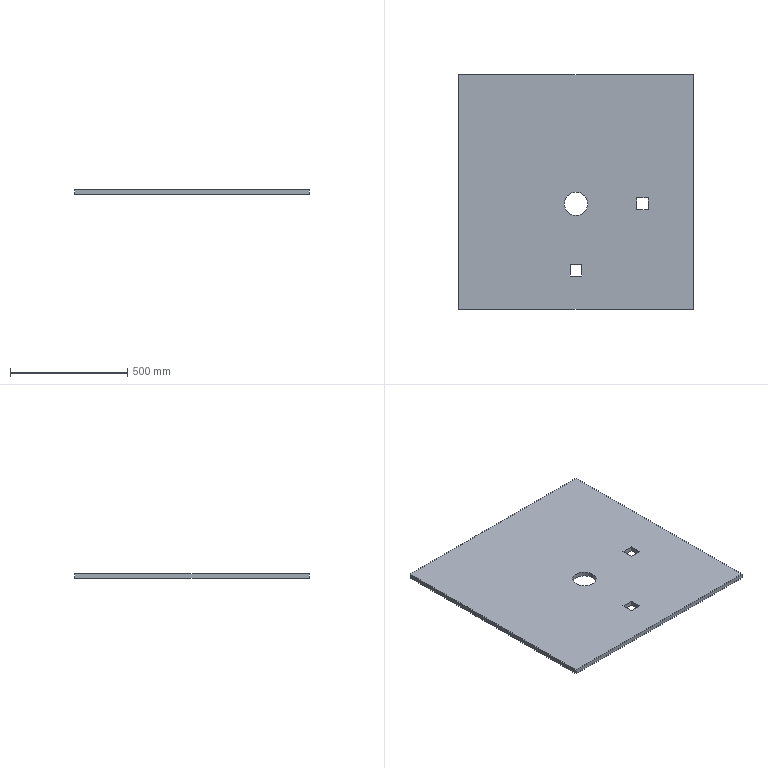Part | STEP file | Large table plate | 1 solid | 16 faces | box 1000 x 1000 x 20 mm | volume 19742920 mm3 | plane 14 | cylinder 2 | commonest cylinder face diameters 100 x2
STEP:
#1=CARTESIAN_POINT('',(0.,0.,0.));
#2=DIRECTION('',(0.,0.,1.));
#3=DIRECTION('',(1.,0.,0.));
#4=AXIS2_PLACEMENT_3D('',#1,#2,#3);
#5=CARTESIAN_POINT('',(50.,-50.,0.));
#6=VERTEX_POINT('',#5);
#7=CARTESIAN_POINT('',(50.,-50.,20.));
#8=VERTEX_POINT('',#7);
#9=CARTESIAN_POINT('',(50.,-50.,0.));
#10=DIRECTION('',(0.,0.,1.));
#11=VECTOR('',#10,1.);
#12=LINE('',#9,#11);
#13=CARTESIAN_POINT('',(0.,-50.,0.));
#14=DIRECTION('',(0.,0.,1.));
#15=DIRECTION('',(1.,0.,0.));
#16=AXIS2_PLACEMENT_3D('',#13,#14,#15);
#17=CYLINDRICAL_SURFACE('',#16,50.);
#18=CARTESIAN_POINT('',(6.283,0.));
#19=DIRECTION('',(0.,1.));
#20=VECTOR('',#19,1.);
#21=LINE('',#18,#20);
#22=(GEOMETRIC_REPRESENTATION_CONTEXT(2)PARAMETRIC_REPRESENTATION_CONTEXT()REPRESENTATION_CONTEXT('',''));
#23=DEFINITIONAL_REPRESENTATION('',(#21),#22);
#24=PCURVE('',#17,#23);
#25=CARTESIAN_POINT('',(0.,-50.,0.));
#26=DIRECTION('',(0.,0.,1.));
#27=DIRECTION('',(1.,0.,0.));
#28=AXIS2_PLACEMENT_3D('',#25,#26,#27);
#29=CYLINDRICAL_SURFACE('',#28,50.);
#30=CARTESIAN_POINT('',(0.,0.));
#31=DIRECTION('',(0.,1.));
#32=VECTOR('',#31,1.);
#33=LINE('',#30,#32);
#34=(GEOMETRIC_REPRESENTATION_CONTEXT(2)PARAMETRIC_REPRESENTATION_CONTEXT()REPRESENTATION_CONTEXT('',''));
#35=DEFINITIONAL_REPRESENTATION('',(#33),#34);
#36=PCURVE('',#29,#35);
#37=SURFACE_CURVE('',#12,(#24,#36),.PCURVE_S1.);
#38=EDGE_CURVE('',#6,#8,#37,.T.);
#39=ORIENTED_EDGE('',*,*,#38,.T.);
#40=CARTESIAN_POINT('',(-50.,-50.,20.));
#41=VERTEX_POINT('',#40);
#42=CARTESIAN_POINT('',(0.,-50.,20.));
#43=DIRECTION('',(0.,0.,-1.));
#44=DIRECTION('',(1.,0.,0.));
#45=AXIS2_PLACEMENT_3D('',#42,#43,#44);
#46=CIRCLE('',#45,50.);
#47=CARTESIAN_POINT('',(6.283,20.));
#48=DIRECTION('',(-1.,0.));
#49=VECTOR('',#48,1.);
#50=LINE('',#47,#49);
#51=(GEOMETRIC_REPRESENTATION_CONTEXT(2)PARAMETRIC_REPRESENTATION_CONTEXT()REPRESENTATION_CONTEXT('',''));
#52=DEFINITIONAL_REPRESENTATION('',(#50),#51);
#53=PCURVE('',#17,#52);
#54=CARTESIAN_POINT('',(0.,0.,20.));
#55=DIRECTION('',(0.,0.,1.));
#56=DIRECTION('',(1.,0.,0.));
#57=AXIS2_PLACEMENT_3D('',#54,#55,#56);
#58=PLANE('',#57);
#59=CARTESIAN_POINT('',(50.,-50.));
#60=CARTESIAN_POINT('',(50.,-136.603));
#61=CARTESIAN_POINT('',(-25.,-93.301));
#62=CARTESIAN_POINT('',(-100.,-50.));
#63=CARTESIAN_POINT('',(-25.,-6.699));
#64=CARTESIAN_POINT('',(50.,36.603));
#65=CARTESIAN_POINT('',(50.,-50.));
#66=(BOUNDED_CURVE()B_SPLINE_CURVE(2,(#59,#60,#61,#62,#63,#64,#65),.UNSPECIFIED.,.T.,.F.)B_SPLINE_CURVE_WITH_KNOTS((1,2,2,2,2,1),(-2.094,0.,2.094,4.189,6.283,8.378),.UNSPECIFIED.)CURVE()GEOMETRIC_REPRESENTATION_ITEM()RATIONAL_B_SPLINE_CURVE((1.,0.5,1.,0.5,1.,0.5,1.))REPRESENTATION_ITEM(''));
#67=(GEOMETRIC_REPRESENTATION_CONTEXT(2)PARAMETRIC_REPRESENTATION_CONTEXT()REPRESENTATION_CONTEXT('',''));
#68=DEFINITIONAL_REPRESENTATION('',(#66),#67);
#69=PCURVE('',#58,#68);
#70=SURFACE_CURVE('',#46,(#53,#69),.PCURVE_S1.);
#71=EDGE_CURVE('',#8,#41,#70,.T.);
#72=ORIENTED_EDGE('',*,*,#71,.T.);
#73=CARTESIAN_POINT('',(-50.,-50.,0.));
#74=VERTEX_POINT('',#73);
#75=CARTESIAN_POINT('',(-50.,-50.,0.));
#76=DIRECTION('',(0.,0.,1.));
#77=VECTOR('',#76,1.);
#78=LINE('',#75,#77);
#79=CARTESIAN_POINT('',(3.142,0.));
#80=DIRECTION('',(0.,1.));
#81=VECTOR('',#80,1.);
#82=LINE('',#79,#81);
#83=(GEOMETRIC_REPRESENTATION_CONTEXT(2)PARAMETRIC_REPRESENTATION_CONTEXT()REPRESENTATION_CONTEXT('',''));
#84=DEFINITIONAL_REPRESENTATION('',(#82),#83);
#85=PCURVE('',#17,#84);
#86=CARTESIAN_POINT('',(3.142,0.));
#87=DIRECTION('',(0.,1.));
#88=VECTOR('',#87,1.);
#89=LINE('',#86,#88);
#90=(GEOMETRIC_REPRESENTATION_CONTEXT(2)PARAMETRIC_REPRESENTATION_CONTEXT()REPRESENTATION_CONTEXT('',''));
#91=DEFINITIONAL_REPRESENTATION('',(#89),#90);
#92=PCURVE('',#29,#91);
#93=SURFACE_CURVE('',#78,(#85,#92),.PCURVE_S1.);
#94=EDGE_CURVE('',#74,#41,#93,.T.);
#95=ORIENTED_EDGE('',*,*,#94,.F.);
#96=CARTESIAN_POINT('',(0.,-50.,0.));
#97=DIRECTION('',(0.,0.,-1.));
#98=DIRECTION('',(1.,0.,0.));
#99=AXIS2_PLACEMENT_3D('',#96,#97,#98);
#100=CIRCLE('',#99,50.);
#101=CARTESIAN_POINT('',(6.283,0.));
#102=DIRECTION('',(-1.,0.));
#103=VECTOR('',#102,1.);
#104=LINE('',#101,#103);
#105=(GEOMETRIC_REPRESENTATION_CONTEXT(2)PARAMETRIC_REPRESENTATION_CONTEXT()REPRESENTATION_CONTEXT('',''));
#106=DEFINITIONAL_REPRESENTATION('',(#104),#105);
#107=PCURVE('',#17,#106);
#108=CARTESIAN_POINT('',(0.,0.,0.));
#109=DIRECTION('',(0.,0.,1.));
#110=DIRECTION('',(1.,0.,0.));
#111=AXIS2_PLACEMENT_3D('',#108,#109,#110);
#112=PLANE('',#111);
#113=CARTESIAN_POINT('',(50.,-50.));
#114=CARTESIAN_POINT('',(50.,-136.603));
#115=CARTESIAN_POINT('',(-25.,-93.301));
#116=CARTESIAN_POINT('',(-100.,-50.));
#117=CARTESIAN_POINT('',(-25.,-6.699));
#118=CARTESIAN_POINT('',(50.,36.603));
#119=CARTESIAN_POINT('',(50.,-50.));
#120=(BOUNDED_CURVE()B_SPLINE_CURVE(2,(#113,#114,#115,#116,#117,#118,#119),.UNSPECIFIED.,.T.,.F.)B_SPLINE_CURVE_WITH_KNOTS((1,2,2,2,2,1),(-2.094,0.,2.094,4.189,6.283,8.378),.UNSPECIFIED.)CURVE()GEOMETRIC_REPRESENTATION_ITEM()RATIONAL_B_SPLINE_CURVE((1.,0.5,1.,0.5,1.,0.5,1.))REPRESENTATION_ITEM(''));
#121=(GEOMETRIC_REPRESENTATION_CONTEXT(2)PARAMETRIC_REPRESENTATION_CONTEXT()REPRESENTATION_CONTEXT('',''));
#122=DEFINITIONAL_REPRESENTATION('',(#120),#121);
#123=PCURVE('',#112,#122);
#124=SURFACE_CURVE('',#100,(#107,#123),.PCURVE_S1.);
#125=EDGE_CURVE('',#6,#74,#124,.T.);
#126=ORIENTED_EDGE('',*,*,#125,.F.);
#127=EDGE_LOOP('',(#39,#72,#95,#126));
#128=FACE_BOUND('',#127,.F.);
#129=ADVANCED_FACE('',(#128),#17,.F.);
#130=CARTESIAN_POINT('',(-500.,-500.,0.));
#131=VERTEX_POINT('',#130);
#132=CARTESIAN_POINT('',(500.,-500.,0.));
#133=VERTEX_POINT('',#132);
#134=CARTESIAN_POINT('',(0.,-500.,0.));
#135=DIRECTION('',(1.,0.,0.));
#136=VECTOR('',#135,1.);
#137=LINE('',#134,#136);
#138=CARTESIAN_POINT('',(0.,-500.));
#139=DIRECTION('',(1.,0.));
#140=VECTOR('',#139,1.);
#141=LINE('',#138,#140);
#142=(GEOMETRIC_REPRESENTATION_CONTEXT(2)PARAMETRIC_REPRESENTATION_CONTEXT()REPRESENTATION_CONTEXT('',''));
#143=DEFINITIONAL_REPRESENTATION('',(#141),#142);
#144=PCURVE('',#112,#143);
#145=CARTESIAN_POINT('',(-500.,-500.,20.));
#146=DIRECTION('',(0.,1.,0.));
#147=DIRECTION('',(0.,0.,1.));
#148=AXIS2_PLACEMENT_3D('',#145,#146,#147);
#149=PLANE('',#148);
#150=CARTESIAN_POINT('',(-20.,500.));
#151=DIRECTION('',(0.,1.));
#152=VECTOR('',#151,1.);
#153=LINE('',#150,#152);
#154=(GEOMETRIC_REPRESENTATION_CONTEXT(2)PARAMETRIC_REPRESENTATION_CONTEXT()REPRESENTATION_CONTEXT('',''));
#155=DEFINITIONAL_REPRESENTATION('',(#153),#154);
#156=PCURVE('',#149,#155);
#157=SURFACE_CURVE('',#137,(#144,#156),.PCURVE_S1.);
#158=EDGE_CURVE('',#131,#133,#157,.T.);
#159=ORIENTED_EDGE('',*,*,#158,.F.);
#160=CARTESIAN_POINT('',(-500.,500.,0.));
#161=VERTEX_POINT('',#160);
#162=CARTESIAN_POINT('',(-500.,0.,0.));
#163=DIRECTION('',(0.,-1.,0.));
#164=VECTOR('',#163,1.);
#165=LINE('',#162,#164);
#166=CARTESIAN_POINT('',(-500.,0.));
#167=DIRECTION('',(0.,-1.));
#168=VECTOR('',#167,1.);
#169=LINE('',#166,#168);
#170=(GEOMETRIC_REPRESENTATION_CONTEXT(2)PARAMETRIC_REPRESENTATION_CONTEXT()REPRESENTATION_CONTEXT('',''));
#171=DEFINITIONAL_REPRESENTATION('',(#169),#170);
#172=PCURVE('',#112,#171);
#173=CARTESIAN_POINT('',(-500.,500.,20.));
#174=DIRECTION('',(1.,0.,0.));
#175=DIRECTION('',(0.,1.,0.));
#176=AXIS2_PLACEMENT_3D('',#173,#174,#175);
#177=PLANE('',#176);
#178=CARTESIAN_POINT('',(-500.,-20.));
#179=DIRECTION('',(-1.,0.));
#180=VECTOR('',#179,1.);
#181=LINE('',#178,#180);
#182=(GEOMETRIC_REPRESENTATION_CONTEXT(2)PARAMETRIC_REPRESENTATION_CONTEXT()REPRESENTATION_CONTEXT('',''));
#183=DEFINITIONAL_REPRESENTATION('',(#181),#182);
#184=PCURVE('',#177,#183);
#185=SURFACE_CURVE('',#165,(#172,#184),.PCURVE_S1.);
#186=EDGE_CURVE('',#161,#131,#185,.T.);
#187=ORIENTED_EDGE('',*,*,#186,.F.);
#188=CARTESIAN_POINT('',(500.,500.,0.));
#189=VERTEX_POINT('',#188);
#190=CARTESIAN_POINT('',(0.,500.,0.));
#191=DIRECTION('',(-1.,0.,0.));
#192=VECTOR('',#191,1.);
#193=LINE('',#190,#192);
#194=CARTESIAN_POINT('',(0.,500.));
#195=DIRECTION('',(-1.,0.));
#196=VECTOR('',#195,1.);
#197=LINE('',#194,#196);
#198=(GEOMETRIC_REPRESENTATION_CONTEXT(2)PARAMETRIC_REPRESENTATION_CONTEXT()REPRESENTATION_CONTEXT('',''));
#199=DEFINITIONAL_REPRESENTATION('',(#197),#198);
#200=PCURVE('',#112,#199);
#201=CARTESIAN_POINT('',(-500.,500.,20.));
#202=DIRECTION('',(0.,-1.,0.));
#203=DIRECTION('',(0.,0.,-1.));
#204=AXIS2_PLACEMENT_3D('',#201,#202,#203);
#205=PLANE('',#204);
#206=CARTESIAN_POINT('',(20.,500.));
#207=DIRECTION('',(0.,-1.));
#208=VECTOR('',#207,1.);
#209=LINE('',#206,#208);
#210=(GEOMETRIC_REPRESENTATION_CONTEXT(2)PARAMETRIC_REPRESENTATION_CONTEXT()REPRESENTATION_CONTEXT('',''));
#211=DEFINITIONAL_REPRESENTATION('',(#209),#210);
#212=PCURVE('',#205,#211);
#213=SURFACE_CURVE('',#193,(#200,#212),.PCURVE_S1.);
#214=EDGE_CURVE('',#189,#161,#213,.T.);
#215=ORIENTED_EDGE('',*,*,#214,.F.);
#216=CARTESIAN_POINT('',(500.,0.,0.));
#217=DIRECTION('',(0.,1.,0.));
#218=VECTOR('',#217,1.);
#219=LINE('',#216,#218);
#220=CARTESIAN_POINT('',(500.,0.));
#221=DIRECTION('',(0.,1.));
#222=VECTOR('',#221,1.);
#223=LINE('',#220,#222);
#224=(GEOMETRIC_REPRESENTATION_CONTEXT(2)PARAMETRIC_REPRESENTATION_CONTEXT()REPRESENTATION_CONTEXT('',''));
#225=DEFINITIONAL_REPRESENTATION('',(#223),#224);
#226=PCURVE('',#112,#225);
#227=CARTESIAN_POINT('',(500.,500.,20.));
#228=DIRECTION('',(-1.,0.,0.));
#229=DIRECTION('',(0.,-1.,0.));
#230=AXIS2_PLACEMENT_3D('',#227,#228,#229);
#231=PLANE('',#230);
#232=CARTESIAN_POINT('',(500.,-20.));
#233=DIRECTION('',(-1.,0.));
#234=VECTOR('',#233,1.);
#235=LINE('',#232,#234);
#236=(GEOMETRIC_REPRESENTATION_CONTEXT(2)PARAMETRIC_REPRESENTATION_CONTEXT()REPRESENTATION_CONTEXT('',''));
#237=DEFINITIONAL_REPRESENTATION('',(#235),#236);
#238=PCURVE('',#231,#237);
#239=SURFACE_CURVE('',#219,(#226,#238),.PCURVE_S1.);
#240=EDGE_CURVE('',#133,#189,#239,.T.);
#241=ORIENTED_EDGE('',*,*,#240,.F.);
#242=EDGE_LOOP('',(#159,#187,#215,#241));
#243=FACE_BOUND('',#242,.T.);
#244=ORIENTED_EDGE('',*,*,#125,.F.);
#245=CARTESIAN_POINT('',(0.,-50.,0.));
#246=DIRECTION('',(0.,0.,-1.));
#247=DIRECTION('',(1.,0.,0.));
#248=AXIS2_PLACEMENT_3D('',#245,#246,#247);
#249=CIRCLE('',#248,50.);
#250=CARTESIAN_POINT('',(50.,-50.));
#251=CARTESIAN_POINT('',(50.,-136.603));
#252=CARTESIAN_POINT('',(-25.,-93.301));
#253=CARTESIAN_POINT('',(-100.,-50.));
#254=CARTESIAN_POINT('',(-25.,-6.699));
#255=CARTESIAN_POINT('',(50.,36.603));
#256=CARTESIAN_POINT('',(50.,-50.));
#257=(BOUNDED_CURVE()B_SPLINE_CURVE(2,(#250,#251,#252,#253,#254,#255,#256),.UNSPECIFIED.,.T.,.F.)B_SPLINE_CURVE_WITH_KNOTS((1,2,2,2,2,1),(-2.094,0.,2.094,4.189,6.283,8.378),.UNSPECIFIED.)CURVE()GEOMETRIC_REPRESENTATION_ITEM()RATIONAL_B_SPLINE_CURVE((1.,0.5,1.,0.5,1.,0.5,1.))REPRESENTATION_ITEM(''));
#258=(GEOMETRIC_REPRESENTATION_CONTEXT(2)PARAMETRIC_REPRESENTATION_CONTEXT()REPRESENTATION_CONTEXT('',''));
#259=DEFINITIONAL_REPRESENTATION('',(#257),#258);
#260=PCURVE('',#112,#259);
#261=CARTESIAN_POINT('',(6.283,0.));
#262=DIRECTION('',(-1.,0.));
#263=VECTOR('',#262,1.);
#264=LINE('',#261,#263);
#265=(GEOMETRIC_REPRESENTATION_CONTEXT(2)PARAMETRIC_REPRESENTATION_CONTEXT()REPRESENTATION_CONTEXT('',''));
#266=DEFINITIONAL_REPRESENTATION('',(#264),#265);
#267=PCURVE('',#29,#266);
#268=SURFACE_CURVE('',#249,(#260,#267),.PCURVE_S1.);
#269=EDGE_CURVE('',#74,#6,#268,.T.);
#270=ORIENTED_EDGE('',*,*,#269,.F.);
#271=EDGE_LOOP('',(#244,#270));
#272=FACE_BOUND('',#271,.T.);
#273=CARTESIAN_POINT('',(308.,-25.,0.));
#274=VERTEX_POINT('',#273);
#275=CARTESIAN_POINT('',(308.,-75.,0.));
#276=VERTEX_POINT('',#275);
#277=CARTESIAN_POINT('',(308.,0.,0.));
#278=DIRECTION('',(0.,-1.,0.));
#279=VECTOR('',#278,1.);
#280=LINE('',#277,#279);
#281=CARTESIAN_POINT('',(308.,0.));
#282=DIRECTION('',(0.,-1.));
#283=VECTOR('',#282,1.);
#284=LINE('',#281,#283);
#285=(GEOMETRIC_REPRESENTATION_CONTEXT(2)PARAMETRIC_REPRESENTATION_CONTEXT()REPRESENTATION_CONTEXT('',''));
#286=DEFINITIONAL_REPRESENTATION('',(#284),#285);
#287=PCURVE('',#112,#286);
#288=CARTESIAN_POINT('',(308.,-25.,30.));
#289=DIRECTION('',(1.,0.,0.));
#290=DIRECTION('',(0.,0.,-1.));
#291=AXIS2_PLACEMENT_3D('',#288,#289,#290);
#292=PLANE('',#291);
#293=CARTESIAN_POINT('',(30.,25.));
#294=DIRECTION('',(0.,-1.));
#295=VECTOR('',#294,1.);
#296=LINE('',#293,#295);
#297=(GEOMETRIC_REPRESENTATION_CONTEXT(2)PARAMETRIC_REPRESENTATION_CONTEXT()REPRESENTATION_CONTEXT('',''));
#298=DEFINITIONAL_REPRESENTATION('',(#296),#297);
#299=PCURVE('',#292,#298);
#300=SURFACE_CURVE('',#280,(#287,#299),.PCURVE_S1.);
#301=EDGE_CURVE('',#274,#276,#300,.T.);
#302=ORIENTED_EDGE('',*,*,#301,.F.);
#303=CARTESIAN_POINT('',(258.,-25.,0.));
#304=VERTEX_POINT('',#303);
#305=CARTESIAN_POINT('',(0.,-25.,0.));
#306=DIRECTION('',(1.,0.,0.));
#307=VECTOR('',#306,1.);
#308=LINE('',#305,#307);
#309=CARTESIAN_POINT('',(0.,-25.));
#310=DIRECTION('',(1.,0.));
#311=VECTOR('',#310,1.);
#312=LINE('',#309,#311);
#313=(GEOMETRIC_REPRESENTATION_CONTEXT(2)PARAMETRIC_REPRESENTATION_CONTEXT()REPRESENTATION_CONTEXT('',''));
#314=DEFINITIONAL_REPRESENTATION('',(#312),#313);
#315=PCURVE('',#112,#314);
#316=CARTESIAN_POINT('',(308.,-25.,30.));
#317=DIRECTION('',(0.,1.,0.));
#318=DIRECTION('',(0.,0.,1.));
#319=AXIS2_PLACEMENT_3D('',#316,#317,#318);
#320=PLANE('',#319);
#321=CARTESIAN_POINT('',(-30.,-308.));
#322=DIRECTION('',(0.,1.));
#323=VECTOR('',#322,1.);
#324=LINE('',#321,#323);
#325=(GEOMETRIC_REPRESENTATION_CONTEXT(2)PARAMETRIC_REPRESENTATION_CONTEXT()REPRESENTATION_CONTEXT('',''));
#326=DEFINITIONAL_REPRESENTATION('',(#324),#325);
#327=PCURVE('',#320,#326);
#328=SURFACE_CURVE('',#308,(#315,#327),.PCURVE_S1.);
#329=EDGE_CURVE('',#304,#274,#328,.T.);
#330=ORIENTED_EDGE('',*,*,#329,.F.);
#331=CARTESIAN_POINT('',(258.,-75.,0.));
#332=VERTEX_POINT('',#331);
#333=CARTESIAN_POINT('',(258.,0.,0.));
#334=DIRECTION('',(0.,1.,0.));
#335=VECTOR('',#334,1.);
#336=LINE('',#333,#335);
#337=CARTESIAN_POINT('',(258.,0.));
#338=DIRECTION('',(0.,1.));
#339=VECTOR('',#338,1.);
#340=LINE('',#337,#339);
#341=(GEOMETRIC_REPRESENTATION_CONTEXT(2)PARAMETRIC_REPRESENTATION_CONTEXT()REPRESENTATION_CONTEXT('',''));
#342=DEFINITIONAL_REPRESENTATION('',(#340),#341);
#343=PCURVE('',#112,#342);
#344=CARTESIAN_POINT('',(258.,-25.,30.));
#345=DIRECTION('',(-1.,0.,0.));
#346=DIRECTION('',(0.,0.,1.));
#347=AXIS2_PLACEMENT_3D('',#344,#345,#346);
#348=PLANE('',#347);
#349=CARTESIAN_POINT('',(-30.,25.));
#350=DIRECTION('',(0.,1.));
#351=VECTOR('',#350,1.);
#352=LINE('',#349,#351);
#353=(GEOMETRIC_REPRESENTATION_CONTEXT(2)PARAMETRIC_REPRESENTATION_CONTEXT()REPRESENTATION_CONTEXT('',''));
#354=DEFINITIONAL_REPRESENTATION('',(#352),#353);
#355=PCURVE('',#348,#354);
#356=SURFACE_CURVE('',#336,(#343,#355),.PCURVE_S1.);
#357=EDGE_CURVE('',#332,#304,#356,.T.);
#358=ORIENTED_EDGE('',*,*,#357,.F.);
#359=CARTESIAN_POINT('',(0.,-75.,0.));
#360=DIRECTION('',(-1.,0.,0.));
#361=VECTOR('',#360,1.);
#362=LINE('',#359,#361);
#363=CARTESIAN_POINT('',(0.,-75.));
#364=DIRECTION('',(-1.,0.));
#365=VECTOR('',#364,1.);
#366=LINE('',#363,#365);
#367=(GEOMETRIC_REPRESENTATION_CONTEXT(2)PARAMETRIC_REPRESENTATION_CONTEXT()REPRESENTATION_CONTEXT('',''));
#368=DEFINITIONAL_REPRESENTATION('',(#366),#367);
#369=PCURVE('',#112,#368);
#370=CARTESIAN_POINT('',(308.,-75.,30.));
#371=DIRECTION('',(0.,-1.,0.));
#372=DIRECTION('',(0.,0.,-1.));
#373=AXIS2_PLACEMENT_3D('',#370,#371,#372);
#374=PLANE('',#373);
#375=CARTESIAN_POINT('',(30.,-308.));
#376=DIRECTION('',(0.,-1.));
#377=VECTOR('',#376,1.);
#378=LINE('',#375,#377);
#379=(GEOMETRIC_REPRESENTATION_CONTEXT(2)PARAMETRIC_REPRESENTATION_CONTEXT()REPRESENTATION_CONTEXT('',''));
#380=DEFINITIONAL_REPRESENTATION('',(#378),#379);
#381=PCURVE('',#374,#380);
#382=SURFACE_CURVE('',#362,(#369,#381),.PCURVE_S1.);
#383=EDGE_CURVE('',#276,#332,#382,.T.);
#384=ORIENTED_EDGE('',*,*,#383,.F.);
#385=EDGE_LOOP('',(#302,#330,#358,#384));
#386=FACE_BOUND('',#385,.T.);
#387=CARTESIAN_POINT('',(25.,-308.,0.));
#388=VERTEX_POINT('',#387);
#389=CARTESIAN_POINT('',(25.,-358.,0.));
#390=VERTEX_POINT('',#389);
#391=CARTESIAN_POINT('',(25.,0.,0.));
#392=DIRECTION('',(0.,-1.,0.));
#393=VECTOR('',#392,1.);
#394=LINE('',#391,#393);
#395=CARTESIAN_POINT('',(25.,0.));
#396=DIRECTION('',(0.,-1.));
#397=VECTOR('',#396,1.);
#398=LINE('',#395,#397);
#399=(GEOMETRIC_REPRESENTATION_CONTEXT(2)PARAMETRIC_REPRESENTATION_CONTEXT()REPRESENTATION_CONTEXT('',''));
#400=DEFINITIONAL_REPRESENTATION('',(#398),#399);
#401=PCURVE('',#112,#400);
#402=CARTESIAN_POINT('',(25.,-308.,30.));
#403=DIRECTION('',(1.,0.,0.));
#404=DIRECTION('',(0.,0.,-1.));
#405=AXIS2_PLACEMENT_3D('',#402,#403,#404);
#406=PLANE('',#405);
#407=CARTESIAN_POINT('',(30.,308.));
#408=DIRECTION('',(0.,-1.));
#409=VECTOR('',#408,1.);
#410=LINE('',#407,#409);
#411=(GEOMETRIC_REPRESENTATION_CONTEXT(2)PARAMETRIC_REPRESENTATION_CONTEXT()REPRESENTATION_CONTEXT('',''));
#412=DEFINITIONAL_REPRESENTATION('',(#410),#411);
#413=PCURVE('',#406,#412);
#414=SURFACE_CURVE('',#394,(#401,#413),.PCURVE_S1.);
#415=EDGE_CURVE('',#388,#390,#414,.T.);
#416=ORIENTED_EDGE('',*,*,#415,.F.);
#417=CARTESIAN_POINT('',(-25.,-308.,0.));
#418=VERTEX_POINT('',#417);
#419=CARTESIAN_POINT('',(0.,-308.,0.));
#420=DIRECTION('',(1.,0.,0.));
#421=VECTOR('',#420,1.);
#422=LINE('',#419,#421);
#423=CARTESIAN_POINT('',(0.,-308.));
#424=DIRECTION('',(1.,0.));
#425=VECTOR('',#424,1.);
#426=LINE('',#423,#425);
#427=(GEOMETRIC_REPRESENTATION_CONTEXT(2)PARAMETRIC_REPRESENTATION_CONTEXT()REPRESENTATION_CONTEXT('',''));
#428=DEFINITIONAL_REPRESENTATION('',(#426),#427);
#429=PCURVE('',#112,#428);
#430=CARTESIAN_POINT('',(25.,-308.,30.));
#431=DIRECTION('',(0.,1.,0.));
#432=DIRECTION('',(0.,0.,1.));
#433=AXIS2_PLACEMENT_3D('',#430,#431,#432);
#434=PLANE('',#433);
#435=CARTESIAN_POINT('',(-30.,-25.));
#436=DIRECTION('',(0.,1.));
#437=VECTOR('',#436,1.);
#438=LINE('',#435,#437);
#439=(GEOMETRIC_REPRESENTATION_CONTEXT(2)PARAMETRIC_REPRESENTATION_CONTEXT()REPRESENTATION_CONTEXT('',''));
#440=DEFINITIONAL_REPRESENTATION('',(#438),#439);
#441=PCURVE('',#434,#440);
#442=SURFACE_CURVE('',#422,(#429,#441),.PCURVE_S1.);
#443=EDGE_CURVE('',#418,#388,#442,.T.);
#444=ORIENTED_EDGE('',*,*,#443,.F.);
#445=CARTESIAN_POINT('',(-25.,-358.,0.));
#446=VERTEX_POINT('',#445);
#447=CARTESIAN_POINT('',(-25.,0.,0.));
#448=DIRECTION('',(0.,1.,0.));
#449=VECTOR('',#448,1.);
#450=LINE('',#447,#449);
#451=CARTESIAN_POINT('',(-25.,0.));
#452=DIRECTION('',(0.,1.));
#453=VECTOR('',#452,1.);
#454=LINE('',#451,#453);
#455=(GEOMETRIC_REPRESENTATION_CONTEXT(2)PARAMETRIC_REPRESENTATION_CONTEXT()REPRESENTATION_CONTEXT('',''));
#456=DEFINITIONAL_REPRESENTATION('',(#454),#455);
#457=PCURVE('',#112,#456);
#458=CARTESIAN_POINT('',(-25.,-308.,30.));
#459=DIRECTION('',(-1.,0.,0.));
#460=DIRECTION('',(0.,0.,1.));
#461=AXIS2_PLACEMENT_3D('',#458,#459,#460);
#462=PLANE('',#461);
#463=CARTESIAN_POINT('',(-30.,308.));
#464=DIRECTION('',(0.,1.));
#465=VECTOR('',#464,1.);
#466=LINE('',#463,#465);
#467=(GEOMETRIC_REPRESENTATION_CONTEXT(2)PARAMETRIC_REPRESENTATION_CONTEXT()REPRESENTATION_CONTEXT('',''));
#468=DEFINITIONAL_REPRESENTATION('',(#466),#467);
#469=PCURVE('',#462,#468);
#470=SURFACE_CURVE('',#450,(#457,#469),.PCURVE_S1.);
#471=EDGE_CURVE('',#446,#418,#470,.T.);
#472=ORIENTED_EDGE('',*,*,#471,.F.);
#473=CARTESIAN_POINT('',(0.,-358.,0.));
#474=DIRECTION('',(-1.,0.,0.));
#475=VECTOR('',#474,1.);
#476=LINE('',#473,#475);
#477=CARTESIAN_POINT('',(0.,-358.));
#478=DIRECTION('',(-1.,0.));
#479=VECTOR('',#478,1.);
#480=LINE('',#477,#479);
#481=(GEOMETRIC_REPRESENTATION_CONTEXT(2)PARAMETRIC_REPRESENTATION_CONTEXT()REPRESENTATION_CONTEXT('',''));
#482=DEFINITIONAL_REPRESENTATION('',(#480),#481);
#483=PCURVE('',#112,#482);
#484=CARTESIAN_POINT('',(25.,-358.,30.));
#485=DIRECTION('',(0.,-1.,0.));
#486=DIRECTION('',(0.,0.,-1.));
#487=AXIS2_PLACEMENT_3D('',#484,#485,#486);
#488=PLANE('',#487);
#489=CARTESIAN_POINT('',(30.,-25.));
#490=DIRECTION('',(0.,-1.));
#491=VECTOR('',#490,1.);
#492=LINE('',#489,#491);
#493=(GEOMETRIC_REPRESENTATION_CONTEXT(2)PARAMETRIC_REPRESENTATION_CONTEXT()REPRESENTATION_CONTEXT('',''));
#494=DEFINITIONAL_REPRESENTATION('',(#492),#493);
#495=PCURVE('',#488,#494);
#496=SURFACE_CURVE('',#476,(#483,#495),.PCURVE_S1.);
#497=EDGE_CURVE('',#390,#446,#496,.T.);
#498=ORIENTED_EDGE('',*,*,#497,.F.);
#499=EDGE_LOOP('',(#416,#444,#472,#498));
#500=FACE_BOUND('',#499,.T.);
#501=ADVANCED_FACE('',(#243,#272,#386,#500),#112,.F.);
#502=CARTESIAN_POINT('',(500.,500.,20.));
#503=VERTEX_POINT('',#502);
#504=CARTESIAN_POINT('',(500.,500.,20.));
#505=DIRECTION('',(0.,0.,-1.));
#506=VECTOR('',#505,1.);
#507=LINE('',#504,#506);
#508=CARTESIAN_POINT('',(0.,0.));
#509=DIRECTION('',(0.,-1.));
#510=VECTOR('',#509,1.);
#511=LINE('',#508,#510);
#512=(GEOMETRIC_REPRESENTATION_CONTEXT(2)PARAMETRIC_REPRESENTATION_CONTEXT()REPRESENTATION_CONTEXT('',''));
#513=DEFINITIONAL_REPRESENTATION('',(#511),#512);
#514=PCURVE('',#231,#513);
#515=CARTESIAN_POINT('',(0.,1000.));
#516=DIRECTION('',(1.,0.));
#517=VECTOR('',#516,1.);
#518=LINE('',#515,#517);
#519=(GEOMETRIC_REPRESENTATION_CONTEXT(2)PARAMETRIC_REPRESENTATION_CONTEXT()REPRESENTATION_CONTEXT('',''));
#520=DEFINITIONAL_REPRESENTATION('',(#518),#519);
#521=PCURVE('',#205,#520);
#522=SURFACE_CURVE('',#507,(#514,#521),.PCURVE_S1.);
#523=EDGE_CURVE('',#503,#189,#522,.T.);
#524=ORIENTED_EDGE('',*,*,#523,.F.);
#525=CARTESIAN_POINT('',(500.,-500.,20.));
#526=VERTEX_POINT('',#525);
#527=CARTESIAN_POINT('',(500.,500.,20.));
#528=DIRECTION('',(0.,1.,0.));
#529=VECTOR('',#528,1.);
#530=LINE('',#527,#529);
#531=CARTESIAN_POINT('',(0.,0.));
#532=DIRECTION('',(-1.,0.));
#533=VECTOR('',#532,1.);
#534=LINE('',#531,#533);
#535=(GEOMETRIC_REPRESENTATION_CONTEXT(2)PARAMETRIC_REPRESENTATION_CONTEXT()REPRESENTATION_CONTEXT('',''));
#536=DEFINITIONAL_REPRESENTATION('',(#534),#535);
#537=PCURVE('',#231,#536);
#538=CARTESIAN_POINT('',(500.,500.));
#539=DIRECTION('',(0.,1.));
#540=VECTOR('',#539,1.);
#541=LINE('',#538,#540);
#542=(GEOMETRIC_REPRESENTATION_CONTEXT(2)PARAMETRIC_REPRESENTATION_CONTEXT()REPRESENTATION_CONTEXT('',''));
#543=DEFINITIONAL_REPRESENTATION('',(#541),#542);
#544=PCURVE('',#58,#543);
#545=SURFACE_CURVE('',#530,(#537,#544),.PCURVE_S1.);
#546=EDGE_CURVE('',#526,#503,#545,.T.);
#547=ORIENTED_EDGE('',*,*,#546,.F.);
#548=CARTESIAN_POINT('',(500.,-500.,20.));
#549=DIRECTION('',(0.,0.,1.));
#550=VECTOR('',#549,1.);
#551=LINE('',#548,#550);
#552=CARTESIAN_POINT('',(1000.,0.));
#553=DIRECTION('',(0.,1.));
#554=VECTOR('',#553,1.);
#555=LINE('',#552,#554);
#556=(GEOMETRIC_REPRESENTATION_CONTEXT(2)PARAMETRIC_REPRESENTATION_CONTEXT()REPRESENTATION_CONTEXT('',''));
#557=DEFINITIONAL_REPRESENTATION('',(#555),#556);
#558=PCURVE('',#231,#557);
#559=CARTESIAN_POINT('',(0.,1000.));
#560=DIRECTION('',(1.,0.));
#561=VECTOR('',#560,1.);
#562=LINE('',#559,#561);
#563=(GEOMETRIC_REPRESENTATION_CONTEXT(2)PARAMETRIC_REPRESENTATION_CONTEXT()REPRESENTATION_CONTEXT('',''));
#564=DEFINITIONAL_REPRESENTATION('',(#562),#563);
#565=PCURVE('',#149,#564);
#566=SURFACE_CURVE('',#551,(#558,#565),.PCURVE_S1.);
#567=EDGE_CURVE('',#133,#526,#566,.T.);
#568=ORIENTED_EDGE('',*,*,#567,.F.);
#569=ORIENTED_EDGE('',*,*,#240,.T.);
#570=EDGE_LOOP('',(#524,#547,#568,#569));
#571=FACE_BOUND('',#570,.T.);
#572=ADVANCED_FACE('',(#571),#231,.F.);
#573=ORIENTED_EDGE('',*,*,#567,.T.);
#574=CARTESIAN_POINT('',(-500.,-500.,20.));
#575=VERTEX_POINT('',#574);
#576=CARTESIAN_POINT('',(-500.,-500.,20.));
#577=DIRECTION('',(1.,0.,0.));
#578=VECTOR('',#577,1.);
#579=LINE('',#576,#578);
#580=CARTESIAN_POINT('',(0.,0.));
#581=DIRECTION('',(0.,1.));
#582=VECTOR('',#581,1.);
#583=LINE('',#580,#582);
#584=(GEOMETRIC_REPRESENTATION_CONTEXT(2)PARAMETRIC_REPRESENTATION_CONTEXT()REPRESENTATION_CONTEXT('',''));
#585=DEFINITIONAL_REPRESENTATION('',(#583),#584);
#586=PCURVE('',#149,#585);
#587=CARTESIAN_POINT('',(-500.,-500.));
#588=DIRECTION('',(1.,0.));
#589=VECTOR('',#588,1.);
#590=LINE('',#587,#589);
#591=(GEOMETRIC_REPRESENTATION_CONTEXT(2)PARAMETRIC_REPRESENTATION_CONTEXT()REPRESENTATION_CONTEXT('',''));
#592=DEFINITIONAL_REPRESENTATION('',(#590),#591);
#593=PCURVE('',#58,#592);
#594=SURFACE_CURVE('',#579,(#586,#593),.PCURVE_S1.);
#595=EDGE_CURVE('',#575,#526,#594,.T.);
#596=ORIENTED_EDGE('',*,*,#595,.F.);
#597=CARTESIAN_POINT('',(-500.,-500.,20.));
#598=DIRECTION('',(0.,0.,1.));
#599=VECTOR('',#598,1.);
#600=LINE('',#597,#599);
#601=CARTESIAN_POINT('',(0.,0.));
#602=DIRECTION('',(1.,0.));
#603=VECTOR('',#602,1.);
#604=LINE('',#601,#603);
#605=(GEOMETRIC_REPRESENTATION_CONTEXT(2)PARAMETRIC_REPRESENTATION_CONTEXT()REPRESENTATION_CONTEXT('',''));
#606=DEFINITIONAL_REPRESENTATION('',(#604),#605);
#607=PCURVE('',#149,#606);
#608=CARTESIAN_POINT('',(-1000.,0.));
#609=DIRECTION('',(0.,1.));
#610=VECTOR('',#609,1.);
#611=LINE('',#608,#610);
#612=(GEOMETRIC_REPRESENTATION_CONTEXT(2)PARAMETRIC_REPRESENTATION_CONTEXT()REPRESENTATION_CONTEXT('',''));
#613=DEFINITIONAL_REPRESENTATION('',(#611),#612);
#614=PCURVE('',#177,#613);
#615=SURFACE_CURVE('',#600,(#607,#614),.PCURVE_S1.);
#616=EDGE_CURVE('',#131,#575,#615,.T.);
#617=ORIENTED_EDGE('',*,*,#616,.F.);
#618=ORIENTED_EDGE('',*,*,#158,.T.);
#619=EDGE_LOOP('',(#573,#596,#617,#618));
#620=FACE_BOUND('',#619,.T.);
#621=ADVANCED_FACE('',(#620),#149,.F.);
#622=ORIENTED_EDGE('',*,*,#616,.T.);
#623=CARTESIAN_POINT('',(-500.,500.,20.));
#624=VERTEX_POINT('',#623);
#625=CARTESIAN_POINT('',(-500.,500.,20.));
#626=DIRECTION('',(0.,-1.,0.));
#627=VECTOR('',#626,1.);
#628=LINE('',#625,#627);
#629=CARTESIAN_POINT('',(0.,0.));
#630=DIRECTION('',(-1.,0.));
#631=VECTOR('',#630,1.);
#632=LINE('',#629,#631);
#633=(GEOMETRIC_REPRESENTATION_CONTEXT(2)PARAMETRIC_REPRESENTATION_CONTEXT()REPRESENTATION_CONTEXT('',''));
#634=DEFINITIONAL_REPRESENTATION('',(#632),#633);
#635=PCURVE('',#177,#634);
#636=CARTESIAN_POINT('',(-500.,500.));
#637=DIRECTION('',(0.,-1.));
#638=VECTOR('',#637,1.);
#639=LINE('',#636,#638);
#640=(GEOMETRIC_REPRESENTATION_CONTEXT(2)PARAMETRIC_REPRESENTATION_CONTEXT()REPRESENTATION_CONTEXT('',''));
#641=DEFINITIONAL_REPRESENTATION('',(#639),#640);
#642=PCURVE('',#58,#641);
#643=SURFACE_CURVE('',#628,(#635,#642),.PCURVE_S1.);
#644=EDGE_CURVE('',#624,#575,#643,.T.);
#645=ORIENTED_EDGE('',*,*,#644,.F.);
#646=CARTESIAN_POINT('',(-500.,500.,20.));
#647=DIRECTION('',(0.,0.,1.));
#648=VECTOR('',#647,1.);
#649=LINE('',#646,#648);
#650=CARTESIAN_POINT('',(0.,0.));
#651=DIRECTION('',(0.,1.));
#652=VECTOR('',#651,1.);
#653=LINE('',#650,#652);
#654=(GEOMETRIC_REPRESENTATION_CONTEXT(2)PARAMETRIC_REPRESENTATION_CONTEXT()REPRESENTATION_CONTEXT('',''));
#655=DEFINITIONAL_REPRESENTATION('',(#653),#654);
#656=PCURVE('',#177,#655);
#657=CARTESIAN_POINT('',(0.,0.));
#658=DIRECTION('',(-1.,0.));
#659=VECTOR('',#658,1.);
#660=LINE('',#657,#659);
#661=(GEOMETRIC_REPRESENTATION_CONTEXT(2)PARAMETRIC_REPRESENTATION_CONTEXT()REPRESENTATION_CONTEXT('',''));
#662=DEFINITIONAL_REPRESENTATION('',(#660),#661);
#663=PCURVE('',#205,#662);
#664=SURFACE_CURVE('',#649,(#656,#663),.PCURVE_S1.);
#665=EDGE_CURVE('',#161,#624,#664,.T.);
#666=ORIENTED_EDGE('',*,*,#665,.F.);
#667=ORIENTED_EDGE('',*,*,#186,.T.);
#668=EDGE_LOOP('',(#622,#645,#666,#667));
#669=FACE_BOUND('',#668,.T.);
#670=ADVANCED_FACE('',(#669),#177,.F.);
#671=ORIENTED_EDGE('',*,*,#665,.T.);
#672=CARTESIAN_POINT('',(-500.,500.,20.));
#673=DIRECTION('',(-1.,0.,0.));
#674=VECTOR('',#673,1.);
#675=LINE('',#672,#674);
#676=CARTESIAN_POINT('',(0.,0.));
#677=DIRECTION('',(0.,-1.));
#678=VECTOR('',#677,1.);
#679=LINE('',#676,#678);
#680=(GEOMETRIC_REPRESENTATION_CONTEXT(2)PARAMETRIC_REPRESENTATION_CONTEXT()REPRESENTATION_CONTEXT('',''));
#681=DEFINITIONAL_REPRESENTATION('',(#679),#680);
#682=PCURVE('',#205,#681);
#683=CARTESIAN_POINT('',(-500.,500.));
#684=DIRECTION('',(-1.,0.));
#685=VECTOR('',#684,1.);
#686=LINE('',#683,#685);
#687=(GEOMETRIC_REPRESENTATION_CONTEXT(2)PARAMETRIC_REPRESENTATION_CONTEXT()REPRESENTATION_CONTEXT('',''));
#688=DEFINITIONAL_REPRESENTATION('',(#686),#687);
#689=PCURVE('',#58,#688);
#690=SURFACE_CURVE('',#675,(#682,#689),.PCURVE_S1.);
#691=EDGE_CURVE('',#503,#624,#690,.T.);
#692=ORIENTED_EDGE('',*,*,#691,.F.);
#693=ORIENTED_EDGE('',*,*,#523,.T.);
#694=ORIENTED_EDGE('',*,*,#214,.T.);
#695=EDGE_LOOP('',(#671,#692,#693,#694));
#696=FACE_BOUND('',#695,.T.);
#697=ADVANCED_FACE('',(#696),#205,.F.);
#698=CARTESIAN_POINT('',(0.,-50.,20.));
#699=DIRECTION('',(0.,0.,-1.));
#700=DIRECTION('',(1.,0.,0.));
#701=AXIS2_PLACEMENT_3D('',#698,#699,#700);
#702=CIRCLE('',#701,50.);
#703=CARTESIAN_POINT('',(6.283,20.));
#704=DIRECTION('',(-1.,0.));
#705=VECTOR('',#704,1.);
#706=LINE('',#703,#705);
#707=(GEOMETRIC_REPRESENTATION_CONTEXT(2)PARAMETRIC_REPRESENTATION_CONTEXT()REPRESENTATION_CONTEXT('',''));
#708=DEFINITIONAL_REPRESENTATION('',(#706),#707);
#709=PCURVE('',#29,#708);
#710=CARTESIAN_POINT('',(50.,-50.));
#711=CARTESIAN_POINT('',(50.,-136.603));
#712=CARTESIAN_POINT('',(-25.,-93.301));
#713=CARTESIAN_POINT('',(-100.,-50.));
#714=CARTESIAN_POINT('',(-25.,-6.699));
#715=CARTESIAN_POINT('',(50.,36.603));
#716=CARTESIAN_POINT('',(50.,-50.));
#717=(BOUNDED_CURVE()B_SPLINE_CURVE(2,(#710,#711,#712,#713,#714,#715,#716),.UNSPECIFIED.,.T.,.F.)B_SPLINE_CURVE_WITH_KNOTS((1,2,2,2,2,1),(-2.094,0.,2.094,4.189,6.283,8.378),.UNSPECIFIED.)CURVE()GEOMETRIC_REPRESENTATION_ITEM()RATIONAL_B_SPLINE_CURVE((1.,0.5,1.,0.5,1.,0.5,1.))REPRESENTATION_ITEM(''));
#718=(GEOMETRIC_REPRESENTATION_CONTEXT(2)PARAMETRIC_REPRESENTATION_CONTEXT()REPRESENTATION_CONTEXT('',''));
#719=DEFINITIONAL_REPRESENTATION('',(#717),#718);
#720=PCURVE('',#58,#719);
#721=SURFACE_CURVE('',#702,(#709,#720),.PCURVE_S1.);
#722=EDGE_CURVE('',#41,#8,#721,.T.);
#723=ORIENTED_EDGE('',*,*,#722,.T.);
#724=ORIENTED_EDGE('',*,*,#38,.F.);
#725=ORIENTED_EDGE('',*,*,#269,.F.);
#726=ORIENTED_EDGE('',*,*,#94,.T.);
#727=EDGE_LOOP('',(#723,#724,#725,#726));
#728=FACE_BOUND('',#727,.F.);
#729=ADVANCED_FACE('',(#728),#29,.F.);
#730=CARTESIAN_POINT('',(308.,-75.,20.));
#731=VERTEX_POINT('',#730);
#732=CARTESIAN_POINT('',(308.,-75.,30.));
#733=DIRECTION('',(0.,0.,1.));
#734=VECTOR('',#733,1.);
#735=LINE('',#732,#734);
#736=CARTESIAN_POINT('',(0.,0.));
#737=DIRECTION('',(-1.,0.));
#738=VECTOR('',#737,1.);
#739=LINE('',#736,#738);
#740=(GEOMETRIC_REPRESENTATION_CONTEXT(2)PARAMETRIC_REPRESENTATION_CONTEXT()REPRESENTATION_CONTEXT('',''));
#741=DEFINITIONAL_REPRESENTATION('',(#739),#740);
#742=PCURVE('',#374,#741);
#743=CARTESIAN_POINT('',(0.,-50.));
#744=DIRECTION('',(-1.,0.));
#745=VECTOR('',#744,1.);
#746=LINE('',#743,#745);
#747=(GEOMETRIC_REPRESENTATION_CONTEXT(2)PARAMETRIC_REPRESENTATION_CONTEXT()REPRESENTATION_CONTEXT('',''));
#748=DEFINITIONAL_REPRESENTATION('',(#746),#747);
#749=PCURVE('',#292,#748);
#750=SURFACE_CURVE('',#735,(#742,#749),.PCURVE_S1.);
#751=EDGE_CURVE('',#276,#731,#750,.T.);
#752=ORIENTED_EDGE('',*,*,#751,.F.);
#753=ORIENTED_EDGE('',*,*,#383,.T.);
#754=CARTESIAN_POINT('',(258.,-75.,20.));
#755=VERTEX_POINT('',#754);
#756=CARTESIAN_POINT('',(258.,-75.,30.));
#757=DIRECTION('',(0.,0.,-1.));
#758=VECTOR('',#757,1.);
#759=LINE('',#756,#758);
#760=CARTESIAN_POINT('',(0.,-50.));
#761=DIRECTION('',(1.,0.));
#762=VECTOR('',#761,1.);
#763=LINE('',#760,#762);
#764=(GEOMETRIC_REPRESENTATION_CONTEXT(2)PARAMETRIC_REPRESENTATION_CONTEXT()REPRESENTATION_CONTEXT('',''));
#765=DEFINITIONAL_REPRESENTATION('',(#763),#764);
#766=PCURVE('',#374,#765);
#767=CARTESIAN_POINT('',(0.,-50.));
#768=DIRECTION('',(-1.,0.));
#769=VECTOR('',#768,1.);
#770=LINE('',#767,#769);
#771=(GEOMETRIC_REPRESENTATION_CONTEXT(2)PARAMETRIC_REPRESENTATION_CONTEXT()REPRESENTATION_CONTEXT('',''));
#772=DEFINITIONAL_REPRESENTATION('',(#770),#771);
#773=PCURVE('',#348,#772);
#774=SURFACE_CURVE('',#759,(#766,#773),.PCURVE_S1.);
#775=EDGE_CURVE('',#755,#332,#774,.T.);
#776=ORIENTED_EDGE('',*,*,#775,.F.);
#777=CARTESIAN_POINT('',(308.,-75.,20.));
#778=DIRECTION('',(-1.,0.,0.));
#779=VECTOR('',#778,1.);
#780=LINE('',#777,#779);
#781=CARTESIAN_POINT('',(10.,0.));
#782=DIRECTION('',(0.,-1.));
#783=VECTOR('',#782,1.);
#784=LINE('',#781,#783);
#785=(GEOMETRIC_REPRESENTATION_CONTEXT(2)PARAMETRIC_REPRESENTATION_CONTEXT()REPRESENTATION_CONTEXT('',''));
#786=DEFINITIONAL_REPRESENTATION('',(#784),#785);
#787=PCURVE('',#374,#786);
#788=CARTESIAN_POINT('',(308.,-75.));
#789=DIRECTION('',(-1.,0.));
#790=VECTOR('',#789,1.);
#791=LINE('',#788,#790);
#792=(GEOMETRIC_REPRESENTATION_CONTEXT(2)PARAMETRIC_REPRESENTATION_CONTEXT()REPRESENTATION_CONTEXT('',''));
#793=DEFINITIONAL_REPRESENTATION('',(#791),#792);
#794=PCURVE('',#58,#793);
#795=SURFACE_CURVE('',#780,(#787,#794),.PCURVE_S1.);
#796=EDGE_CURVE('',#731,#755,#795,.T.);
#797=ORIENTED_EDGE('',*,*,#796,.F.);
#798=EDGE_LOOP('',(#752,#753,#776,#797));
#799=FACE_BOUND('',#798,.T.);
#800=ADVANCED_FACE('',(#799),#374,.F.);
#801=CARTESIAN_POINT('',(308.,-25.,20.));
#802=VERTEX_POINT('',#801);
#803=CARTESIAN_POINT('',(308.,-25.,30.));
#804=DIRECTION('',(0.,0.,1.));
#805=VECTOR('',#804,1.);
#806=LINE('',#803,#805);
#807=CARTESIAN_POINT('',(0.,0.));
#808=DIRECTION('',(-1.,0.));
#809=VECTOR('',#808,1.);
#810=LINE('',#807,#809);
#811=(GEOMETRIC_REPRESENTATION_CONTEXT(2)PARAMETRIC_REPRESENTATION_CONTEXT()REPRESENTATION_CONTEXT('',''));
#812=DEFINITIONAL_REPRESENTATION('',(#810),#811);
#813=PCURVE('',#292,#812);
#814=CARTESIAN_POINT('',(0.,0.));
#815=DIRECTION('',(1.,0.));
#816=VECTOR('',#815,1.);
#817=LINE('',#814,#816);
#818=(GEOMETRIC_REPRESENTATION_CONTEXT(2)PARAMETRIC_REPRESENTATION_CONTEXT()REPRESENTATION_CONTEXT('',''));
#819=DEFINITIONAL_REPRESENTATION('',(#817),#818);
#820=PCURVE('',#320,#819);
#821=SURFACE_CURVE('',#806,(#813,#820),.PCURVE_S1.);
#822=EDGE_CURVE('',#274,#802,#821,.T.);
#823=ORIENTED_EDGE('',*,*,#822,.F.);
#824=ORIENTED_EDGE('',*,*,#301,.T.);
#825=ORIENTED_EDGE('',*,*,#751,.T.);
#826=CARTESIAN_POINT('',(308.,-25.,20.));
#827=DIRECTION('',(0.,-1.,0.));
#828=VECTOR('',#827,1.);
#829=LINE('',#826,#828);
#830=CARTESIAN_POINT('',(10.,0.));
#831=DIRECTION('',(0.,-1.));
#832=VECTOR('',#831,1.);
#833=LINE('',#830,#832);
#834=(GEOMETRIC_REPRESENTATION_CONTEXT(2)PARAMETRIC_REPRESENTATION_CONTEXT()REPRESENTATION_CONTEXT('',''));
#835=DEFINITIONAL_REPRESENTATION('',(#833),#834);
#836=PCURVE('',#292,#835);
#837=CARTESIAN_POINT('',(308.,-25.));
#838=DIRECTION('',(0.,-1.));
#839=VECTOR('',#838,1.);
#840=LINE('',#837,#839);
#841=(GEOMETRIC_REPRESENTATION_CONTEXT(2)PARAMETRIC_REPRESENTATION_CONTEXT()REPRESENTATION_CONTEXT('',''));
#842=DEFINITIONAL_REPRESENTATION('',(#840),#841);
#843=PCURVE('',#58,#842);
#844=SURFACE_CURVE('',#829,(#836,#843),.PCURVE_S1.);
#845=EDGE_CURVE('',#802,#731,#844,.T.);
#846=ORIENTED_EDGE('',*,*,#845,.F.);
#847=EDGE_LOOP('',(#823,#824,#825,#846));
#848=FACE_BOUND('',#847,.T.);
#849=ADVANCED_FACE('',(#848),#292,.F.);
#850=CARTESIAN_POINT('',(258.,-25.,20.));
#851=VERTEX_POINT('',#850);
#852=CARTESIAN_POINT('',(258.,-25.,30.));
#853=DIRECTION('',(0.,0.,1.));
#854=VECTOR('',#853,1.);
#855=LINE('',#852,#854);
#856=CARTESIAN_POINT('',(0.,-50.));
#857=DIRECTION('',(1.,0.));
#858=VECTOR('',#857,1.);
#859=LINE('',#856,#858);
#860=(GEOMETRIC_REPRESENTATION_CONTEXT(2)PARAMETRIC_REPRESENTATION_CONTEXT()REPRESENTATION_CONTEXT('',''));
#861=DEFINITIONAL_REPRESENTATION('',(#859),#860);
#862=PCURVE('',#320,#861);
#863=CARTESIAN_POINT('',(0.,0.));
#864=DIRECTION('',(1.,0.));
#865=VECTOR('',#864,1.);
#866=LINE('',#863,#865);
#867=(GEOMETRIC_REPRESENTATION_CONTEXT(2)PARAMETRIC_REPRESENTATION_CONTEXT()REPRESENTATION_CONTEXT('',''));
#868=DEFINITIONAL_REPRESENTATION('',(#866),#867);
#869=PCURVE('',#348,#868);
#870=SURFACE_CURVE('',#855,(#862,#869),.PCURVE_S1.);
#871=EDGE_CURVE('',#304,#851,#870,.T.);
#872=ORIENTED_EDGE('',*,*,#871,.F.);
#873=ORIENTED_EDGE('',*,*,#329,.T.);
#874=ORIENTED_EDGE('',*,*,#822,.T.);
#875=CARTESIAN_POINT('',(308.,-25.,20.));
#876=DIRECTION('',(1.,0.,0.));
#877=VECTOR('',#876,1.);
#878=LINE('',#875,#877);
#879=CARTESIAN_POINT('',(-10.,0.));
#880=DIRECTION('',(0.,1.));
#881=VECTOR('',#880,1.);
#882=LINE('',#879,#881);
#883=(GEOMETRIC_REPRESENTATION_CONTEXT(2)PARAMETRIC_REPRESENTATION_CONTEXT()REPRESENTATION_CONTEXT('',''));
#884=DEFINITIONAL_REPRESENTATION('',(#882),#883);
#885=PCURVE('',#320,#884);
#886=CARTESIAN_POINT('',(308.,-25.));
#887=DIRECTION('',(1.,0.));
#888=VECTOR('',#887,1.);
#889=LINE('',#886,#888);
#890=(GEOMETRIC_REPRESENTATION_CONTEXT(2)PARAMETRIC_REPRESENTATION_CONTEXT()REPRESENTATION_CONTEXT('',''));
#891=DEFINITIONAL_REPRESENTATION('',(#889),#890);
#892=PCURVE('',#58,#891);
#893=SURFACE_CURVE('',#878,(#885,#892),.PCURVE_S1.);
#894=EDGE_CURVE('',#851,#802,#893,.T.);
#895=ORIENTED_EDGE('',*,*,#894,.F.);
#896=EDGE_LOOP('',(#872,#873,#874,#895));
#897=FACE_BOUND('',#896,.T.);
#898=ADVANCED_FACE('',(#897),#320,.F.);
#899=ORIENTED_EDGE('',*,*,#775,.T.);
#900=ORIENTED_EDGE('',*,*,#357,.T.);
#901=ORIENTED_EDGE('',*,*,#871,.T.);
#902=CARTESIAN_POINT('',(258.,-25.,20.));
#903=DIRECTION('',(0.,1.,0.));
#904=VECTOR('',#903,1.);
#905=LINE('',#902,#904);
#906=CARTESIAN_POINT('',(-10.,0.));
#907=DIRECTION('',(0.,1.));
#908=VECTOR('',#907,1.);
#909=LINE('',#906,#908);
#910=(GEOMETRIC_REPRESENTATION_CONTEXT(2)PARAMETRIC_REPRESENTATION_CONTEXT()REPRESENTATION_CONTEXT('',''));
#911=DEFINITIONAL_REPRESENTATION('',(#909),#910);
#912=PCURVE('',#348,#911);
#913=CARTESIAN_POINT('',(258.,-25.));
#914=DIRECTION('',(0.,1.));
#915=VECTOR('',#914,1.);
#916=LINE('',#913,#915);
#917=(GEOMETRIC_REPRESENTATION_CONTEXT(2)PARAMETRIC_REPRESENTATION_CONTEXT()REPRESENTATION_CONTEXT('',''));
#918=DEFINITIONAL_REPRESENTATION('',(#916),#917);
#919=PCURVE('',#58,#918);
#920=SURFACE_CURVE('',#905,(#912,#919),.PCURVE_S1.);
#921=EDGE_CURVE('',#755,#851,#920,.T.);
#922=ORIENTED_EDGE('',*,*,#921,.F.);
#923=EDGE_LOOP('',(#899,#900,#901,#922));
#924=FACE_BOUND('',#923,.T.);
#925=ADVANCED_FACE('',(#924),#348,.F.);
#926=CARTESIAN_POINT('',(25.,-358.,20.));
#927=VERTEX_POINT('',#926);
#928=CARTESIAN_POINT('',(25.,-358.,30.));
#929=DIRECTION('',(0.,0.,1.));
#930=VECTOR('',#929,1.);
#931=LINE('',#928,#930);
#932=CARTESIAN_POINT('',(0.,0.));
#933=DIRECTION('',(-1.,0.));
#934=VECTOR('',#933,1.);
#935=LINE('',#932,#934);
#936=(GEOMETRIC_REPRESENTATION_CONTEXT(2)PARAMETRIC_REPRESENTATION_CONTEXT()REPRESENTATION_CONTEXT('',''));
#937=DEFINITIONAL_REPRESENTATION('',(#935),#936);
#938=PCURVE('',#488,#937);
#939=CARTESIAN_POINT('',(0.,-50.));
#940=DIRECTION('',(-1.,0.));
#941=VECTOR('',#940,1.);
#942=LINE('',#939,#941);
#943=(GEOMETRIC_REPRESENTATION_CONTEXT(2)PARAMETRIC_REPRESENTATION_CONTEXT()REPRESENTATION_CONTEXT('',''));
#944=DEFINITIONAL_REPRESENTATION('',(#942),#943);
#945=PCURVE('',#406,#944);
#946=SURFACE_CURVE('',#931,(#938,#945),.PCURVE_S1.);
#947=EDGE_CURVE('',#390,#927,#946,.T.);
#948=ORIENTED_EDGE('',*,*,#947,.F.);
#949=ORIENTED_EDGE('',*,*,#497,.T.);
#950=CARTESIAN_POINT('',(-25.,-358.,20.));
#951=VERTEX_POINT('',#950);
#952=CARTESIAN_POINT('',(-25.,-358.,30.));
#953=DIRECTION('',(0.,0.,-1.));
#954=VECTOR('',#953,1.);
#955=LINE('',#952,#954);
#956=CARTESIAN_POINT('',(0.,-50.));
#957=DIRECTION('',(1.,0.));
#958=VECTOR('',#957,1.);
#959=LINE('',#956,#958);
#960=(GEOMETRIC_REPRESENTATION_CONTEXT(2)PARAMETRIC_REPRESENTATION_CONTEXT()REPRESENTATION_CONTEXT('',''));
#961=DEFINITIONAL_REPRESENTATION('',(#959),#960);
#962=PCURVE('',#488,#961);
#963=CARTESIAN_POINT('',(0.,-50.));
#964=DIRECTION('',(-1.,0.));
#965=VECTOR('',#964,1.);
#966=LINE('',#963,#965);
#967=(GEOMETRIC_REPRESENTATION_CONTEXT(2)PARAMETRIC_REPRESENTATION_CONTEXT()REPRESENTATION_CONTEXT('',''));
#968=DEFINITIONAL_REPRESENTATION('',(#966),#967);
#969=PCURVE('',#462,#968);
#970=SURFACE_CURVE('',#955,(#962,#969),.PCURVE_S1.);
#971=EDGE_CURVE('',#951,#446,#970,.T.);
#972=ORIENTED_EDGE('',*,*,#971,.F.);
#973=CARTESIAN_POINT('',(25.,-358.,20.));
#974=DIRECTION('',(-1.,0.,0.));
#975=VECTOR('',#974,1.);
#976=LINE('',#973,#975);
#977=CARTESIAN_POINT('',(10.,0.));
#978=DIRECTION('',(0.,-1.));
#979=VECTOR('',#978,1.);
#980=LINE('',#977,#979);
#981=(GEOMETRIC_REPRESENTATION_CONTEXT(2)PARAMETRIC_REPRESENTATION_CONTEXT()REPRESENTATION_CONTEXT('',''));
#982=DEFINITIONAL_REPRESENTATION('',(#980),#981);
#983=PCURVE('',#488,#982);
#984=CARTESIAN_POINT('',(25.,-358.));
#985=DIRECTION('',(-1.,0.));
#986=VECTOR('',#985,1.);
#987=LINE('',#984,#986);
#988=(GEOMETRIC_REPRESENTATION_CONTEXT(2)PARAMETRIC_REPRESENTATION_CONTEXT()REPRESENTATION_CONTEXT('',''));
#989=DEFINITIONAL_REPRESENTATION('',(#987),#988);
#990=PCURVE('',#58,#989);
#991=SURFACE_CURVE('',#976,(#983,#990),.PCURVE_S1.);
#992=EDGE_CURVE('',#927,#951,#991,.T.);
#993=ORIENTED_EDGE('',*,*,#992,.F.);
#994=EDGE_LOOP('',(#948,#949,#972,#993));
#995=FACE_BOUND('',#994,.T.);
#996=ADVANCED_FACE('',(#995),#488,.F.);
#997=CARTESIAN_POINT('',(25.,-308.,20.));
#998=VERTEX_POINT('',#997);
#999=CARTESIAN_POINT('',(25.,-308.,30.));
#1000=DIRECTION('',(0.,0.,1.));
#1001=VECTOR('',#1000,1.);
#1002=LINE('',#999,#1001);
#1003=CARTESIAN_POINT('',(0.,0.));
#1004=DIRECTION('',(-1.,0.));
#1005=VECTOR('',#1004,1.);
#1006=LINE('',#1003,#1005);
#1007=(GEOMETRIC_REPRESENTATION_CONTEXT(2)PARAMETRIC_REPRESENTATION_CONTEXT()REPRESENTATION_CONTEXT('',''));
#1008=DEFINITIONAL_REPRESENTATION('',(#1006),#1007);
#1009=PCURVE('',#406,#1008);
#1010=CARTESIAN_POINT('',(0.,0.));
#1011=DIRECTION('',(1.,0.));
#1012=VECTOR('',#1011,1.);
#1013=LINE('',#1010,#1012);
#1014=(GEOMETRIC_REPRESENTATION_CONTEXT(2)PARAMETRIC_REPRESENTATION_CONTEXT()REPRESENTATION_CONTEXT('',''));
#1015=DEFINITIONAL_REPRESENTATION('',(#1013),#1014);
#1016=PCURVE('',#434,#1015);
#1017=SURFACE_CURVE('',#1002,(#1009,#1016),.PCURVE_S1.);
#1018=EDGE_CURVE('',#388,#998,#1017,.T.);
#1019=ORIENTED_EDGE('',*,*,#1018,.F.);
#1020=ORIENTED_EDGE('',*,*,#415,.T.);
#1021=ORIENTED_EDGE('',*,*,#947,.T.);
#1022=CARTESIAN_POINT('',(25.,-308.,20.));
#1023=DIRECTION('',(0.,-1.,0.));
#1024=VECTOR('',#1023,1.);
#1025=LINE('',#1022,#1024);
#1026=CARTESIAN_POINT('',(10.,0.));
#1027=DIRECTION('',(0.,-1.));
#1028=VECTOR('',#1027,1.);
#1029=LINE('',#1026,#1028);
#1030=(GEOMETRIC_REPRESENTATION_CONTEXT(2)PARAMETRIC_REPRESENTATION_CONTEXT()REPRESENTATION_CONTEXT('',''));
#1031=DEFINITIONAL_REPRESENTATION('',(#1029),#1030);
#1032=PCURVE('',#406,#1031);
#1033=CARTESIAN_POINT('',(25.,-308.));
#1034=DIRECTION('',(0.,-1.));
#1035=VECTOR('',#1034,1.);
#1036=LINE('',#1033,#1035);
#1037=(GEOMETRIC_REPRESENTATION_CONTEXT(2)PARAMETRIC_REPRESENTATION_CONTEXT()REPRESENTATION_CONTEXT('',''));
#1038=DEFINITIONAL_REPRESENTATION('',(#1036),#1037);
#1039=PCURVE('',#58,#1038);
#1040=SURFACE_CURVE('',#1025,(#1032,#1039),.PCURVE_S1.);
#1041=EDGE_CURVE('',#998,#927,#1040,.T.);
#1042=ORIENTED_EDGE('',*,*,#1041,.F.);
#1043=EDGE_LOOP('',(#1019,#1020,#1021,#1042));
#1044=FACE_BOUND('',#1043,.T.);
#1045=ADVANCED_FACE('',(#1044),#406,.F.);
#1046=CARTESIAN_POINT('',(-25.,-308.,20.));
#1047=VERTEX_POINT('',#1046);
#1048=CARTESIAN_POINT('',(-25.,-308.,30.));
#1049=DIRECTION('',(0.,0.,1.));
#1050=VECTOR('',#1049,1.);
#1051=LINE('',#1048,#1050);
#1052=CARTESIAN_POINT('',(0.,-50.));
#1053=DIRECTION('',(1.,0.));
#1054=VECTOR('',#1053,1.);
#1055=LINE('',#1052,#1054);
#1056=(GEOMETRIC_REPRESENTATION_CONTEXT(2)PARAMETRIC_REPRESENTATION_CONTEXT()REPRESENTATION_CONTEXT('',''));
#1057=DEFINITIONAL_REPRESENTATION('',(#1055),#1056);
#1058=PCURVE('',#434,#1057);
#1059=CARTESIAN_POINT('',(0.,0.));
#1060=DIRECTION('',(1.,0.));
#1061=VECTOR('',#1060,1.);
#1062=LINE('',#1059,#1061);
#1063=(GEOMETRIC_REPRESENTATION_CONTEXT(2)PARAMETRIC_REPRESENTATION_CONTEXT()REPRESENTATION_CONTEXT('',''));
#1064=DEFINITIONAL_REPRESENTATION('',(#1062),#1063);
#1065=PCURVE('',#462,#1064);
#1066=SURFACE_CURVE('',#1051,(#1058,#1065),.PCURVE_S1.);
#1067=EDGE_CURVE('',#418,#1047,#1066,.T.);
#1068=ORIENTED_EDGE('',*,*,#1067,.F.);
#1069=ORIENTED_EDGE('',*,*,#443,.T.);
#1070=ORIENTED_EDGE('',*,*,#1018,.T.);
#1071=CARTESIAN_POINT('',(25.,-308.,20.));
#1072=DIRECTION('',(1.,0.,0.));
#1073=VECTOR('',#1072,1.);
#1074=LINE('',#1071,#1073);
#1075=CARTESIAN_POINT('',(-10.,0.));
#1076=DIRECTION('',(0.,1.));
#1077=VECTOR('',#1076,1.);
#1078=LINE('',#1075,#1077);
#1079=(GEOMETRIC_REPRESENTATION_CONTEXT(2)PARAMETRIC_REPRESENTATION_CONTEXT()REPRESENTATION_CONTEXT('',''));
#1080=DEFINITIONAL_REPRESENTATION('',(#1078),#1079);
#1081=PCURVE('',#434,#1080);
#1082=CARTESIAN_POINT('',(25.,-308.));
#1083=DIRECTION('',(1.,0.));
#1084=VECTOR('',#1083,1.);
#1085=LINE('',#1082,#1084);
#1086=(GEOMETRIC_REPRESENTATION_CONTEXT(2)PARAMETRIC_REPRESENTATION_CONTEXT()REPRESENTATION_CONTEXT('',''));
#1087=DEFINITIONAL_REPRESENTATION('',(#1085),#1086);
#1088=PCURVE('',#58,#1087);
#1089=SURFACE_CURVE('',#1074,(#1081,#1088),.PCURVE_S1.);
#1090=EDGE_CURVE('',#1047,#998,#1089,.T.);
#1091=ORIENTED_EDGE('',*,*,#1090,.F.);
#1092=EDGE_LOOP('',(#1068,#1069,#1070,#1091));
#1093=FACE_BOUND('',#1092,.T.);
#1094=ADVANCED_FACE('',(#1093),#434,.F.);
#1095=ORIENTED_EDGE('',*,*,#971,.T.);
#1096=ORIENTED_EDGE('',*,*,#471,.T.);
#1097=ORIENTED_EDGE('',*,*,#1067,.T.);
#1098=CARTESIAN_POINT('',(-25.,-308.,20.));
#1099=DIRECTION('',(0.,1.,0.));
#1100=VECTOR('',#1099,1.);
#1101=LINE('',#1098,#1100);
#1102=CARTESIAN_POINT('',(-10.,0.));
#1103=DIRECTION('',(0.,1.));
#1104=VECTOR('',#1103,1.);
#1105=LINE('',#1102,#1104);
#1106=(GEOMETRIC_REPRESENTATION_CONTEXT(2)PARAMETRIC_REPRESENTATION_CONTEXT()REPRESENTATION_CONTEXT('',''));
#1107=DEFINITIONAL_REPRESENTATION('',(#1105),#1106);
#1108=PCURVE('',#462,#1107);
#1109=CARTESIAN_POINT('',(-25.,-308.));
#1110=DIRECTION('',(0.,1.));
#1111=VECTOR('',#1110,1.);
#1112=LINE('',#1109,#1111);
#1113=(GEOMETRIC_REPRESENTATION_CONTEXT(2)PARAMETRIC_REPRESENTATION_CONTEXT()REPRESENTATION_CONTEXT('',''));
#1114=DEFINITIONAL_REPRESENTATION('',(#1112),#1113);
#1115=PCURVE('',#58,#1114);
#1116=SURFACE_CURVE('',#1101,(#1108,#1115),.PCURVE_S1.);
#1117=EDGE_CURVE('',#951,#1047,#1116,.T.);
#1118=ORIENTED_EDGE('',*,*,#1117,.F.);
#1119=EDGE_LOOP('',(#1095,#1096,#1097,#1118));
#1120=FACE_BOUND('',#1119,.T.);
#1121=ADVANCED_FACE('',(#1120),#462,.F.);
#1122=ORIENTED_EDGE('',*,*,#644,.T.);
#1123=ORIENTED_EDGE('',*,*,#595,.T.);
#1124=ORIENTED_EDGE('',*,*,#546,.T.);
#1125=ORIENTED_EDGE('',*,*,#691,.T.);
#1126=EDGE_LOOP('',(#1122,#1123,#1124,#1125));
#1127=FACE_BOUND('',#1126,.T.);
#1128=ORIENTED_EDGE('',*,*,#71,.T.);
#1129=ORIENTED_EDGE('',*,*,#722,.T.);
#1130=EDGE_LOOP('',(#1128,#1129));
#1131=FACE_BOUND('',#1130,.T.);
#1132=ORIENTED_EDGE('',*,*,#921,.T.);
#1133=ORIENTED_EDGE('',*,*,#894,.T.);
#1134=ORIENTED_EDGE('',*,*,#845,.T.);
#1135=ORIENTED_EDGE('',*,*,#796,.T.);
#1136=EDGE_LOOP('',(#1132,#1133,#1134,#1135));
#1137=FACE_BOUND('',#1136,.T.);
#1138=ORIENTED_EDGE('',*,*,#1117,.T.);
#1139=ORIENTED_EDGE('',*,*,#1090,.T.);
#1140=ORIENTED_EDGE('',*,*,#1041,.T.);
#1141=ORIENTED_EDGE('',*,*,#992,.T.);
#1142=EDGE_LOOP('',(#1138,#1139,#1140,#1141));
#1143=FACE_BOUND('',#1142,.T.);
#1144=ADVANCED_FACE('',(#1127,#1131,#1137,#1143),#58,.T.);
#1145=CLOSED_SHELL('',(#129,#501,#572,#621,#670,#697,#729,#800,#849,#898,#925,#996,#1045,#1094,#1121,#1144));
#1146=MANIFOLD_SOLID_BREP('',#1145);
#1147=(LENGTH_UNIT()NAMED_UNIT(*)SI_UNIT(.MILLI.,.METRE.));
#1148=UNCERTAINTY_MEASURE_WITH_UNIT(LENGTH_MEASURE(0.0000001),#1147,'','');
#1149=(NAMED_UNIT(*)PLANE_ANGLE_UNIT()SI_UNIT($,.RADIAN.));
#1150=(NAMED_UNIT(*)SI_UNIT($,.STERADIAN.)SOLID_ANGLE_UNIT());
#1151=(GEOMETRIC_REPRESENTATION_CONTEXT(3)GLOBAL_UNCERTAINTY_ASSIGNED_CONTEXT((#1148))GLOBAL_UNIT_ASSIGNED_CONTEXT((#1147,#1149,#1150))REPRESENTATION_CONTEXT('',''));
#1152=ADVANCED_BREP_SHAPE_REPRESENTATION('',(#4,#1146),#1151);